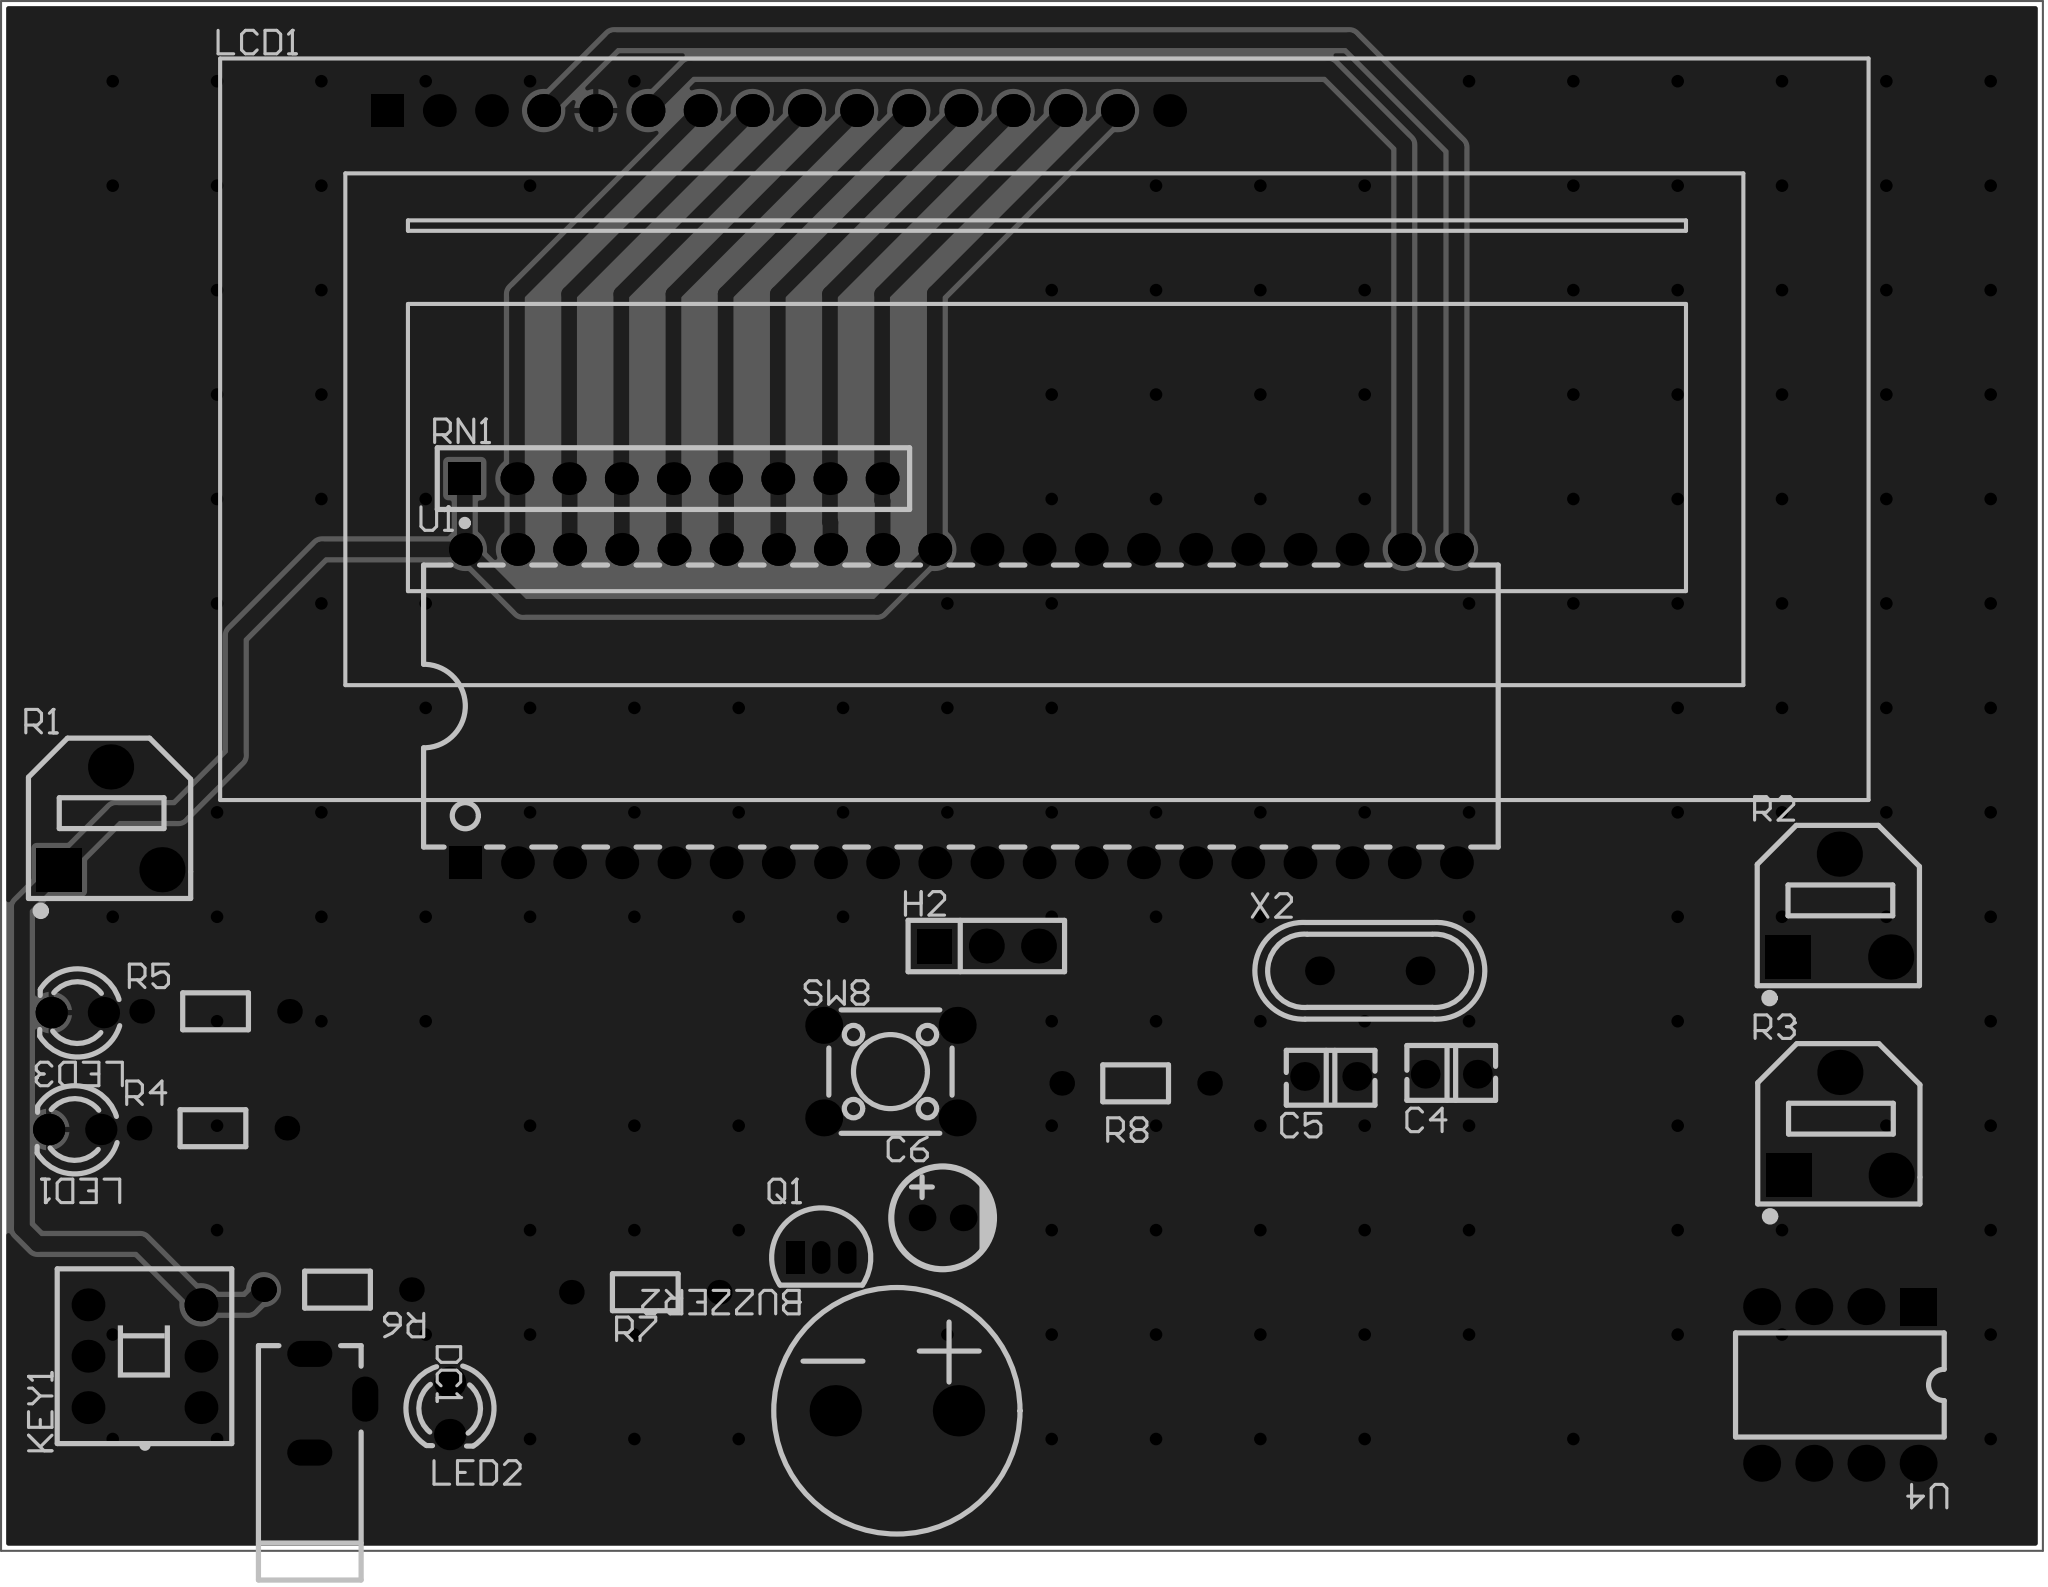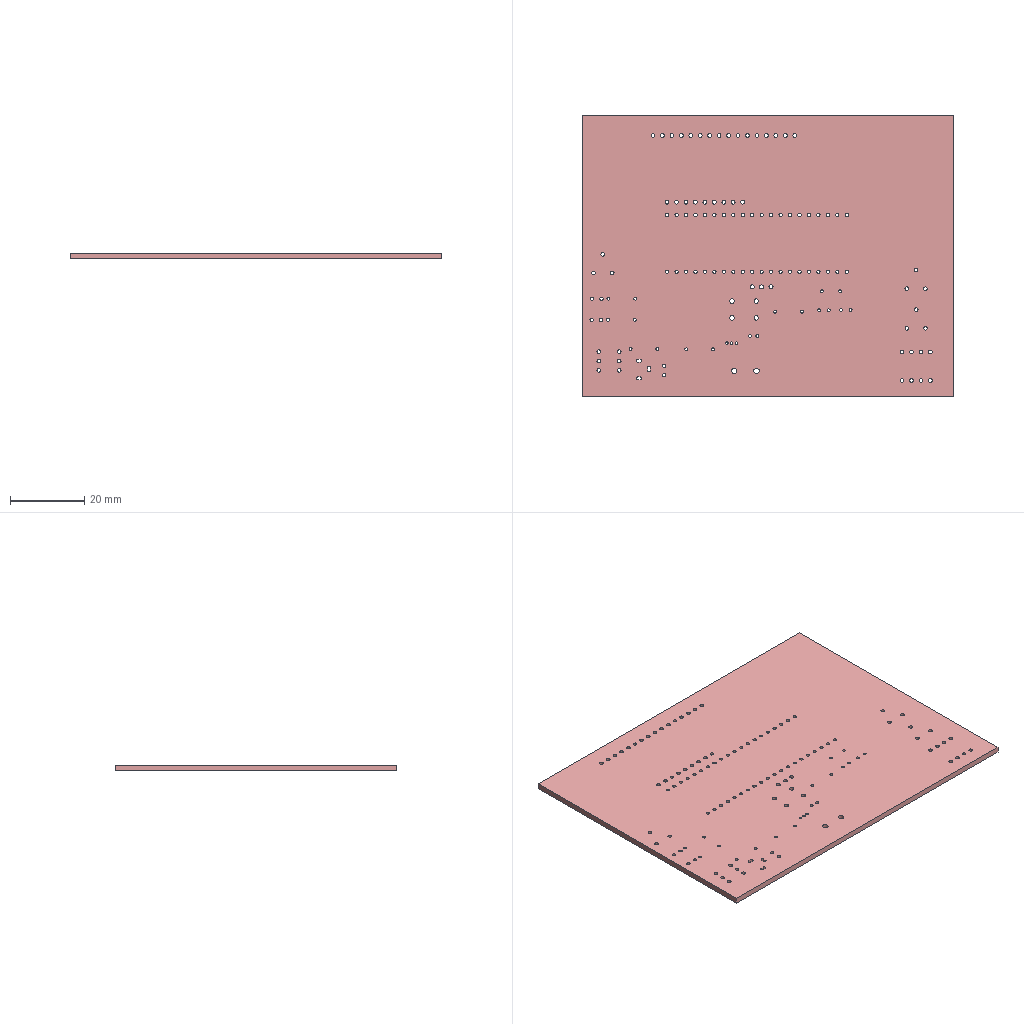Circuit board layout | Altium Designer | box 99.4 x 75.4 x 1.6 mm
Layer stack:
# Altium Designer layer stack of  (unit mm; dielectric type: 0 none, 1 core, 2 prepreg, 3 surface material)
index,name,kind,layer,copper_thickness_mm,dielectric_type,dielectric_thickness_mm,dielectric_material,dielectric_constant
0,Top Paste Mask Layer,other,,,,,,
1,Top Silkscreen Layer,other,,,,,,
2,Top Solder Mask Layer,dielectric,,,3,0.01,,3.3
3,Top Layer,copper,Top Layer,0.035,,,,
4,Dielectric1,dielectric,,,3,1.51,FR4,4.5
5,Bottom Layer,copper,Bottom Layer,0.035,,,,
6,Bottom Solder Mask Layer,dielectric,,,3,0.01,,3.3
7,Bottom Silkscreen Layer,other,,,,,,
8,Bottom Paste Mask Layer,other,,,,,,
# drill layer pairs: low layer,high layer
drill_pair,Top Layer,Bottom Layer
Part placement:
Designator,Comment,Layer,Footprint,Center-X(mm),Center-Y(mm),Rotation
BUZZER2,buzzer,TopLayer,BUZ-TH_BD12.0-P6.00-D0.9-RD,137.346,90.057,0
C4,30pF,TopLayer,CAP-TH_L3.8-W2.5-P2.54-D0.50,164.338,106.426,180
C5,30pF,TopLayer,CAP-TH_L3.8-W2.5-P2.54-D0.50,158.466,106.317,0
C6,10uF,TopLayer,CAP-TH_BD5.0-P2.00-D0.8-FD-10UF50VC110GL,139.573,99.441,0
H2,,TopLayer,HDR-TH_3P-P2.54-V-M,141.702,112.661,0
KEY1,无自锁开关 8.5×8.5 无声,TopLayer,SW-TH_6P-L8.5-W8.5-P2.54,100.711,92.71,90
LCD1,LCD1602,TopLayer,LCD1602,131.576,153.295,0
LED2,,TopLayer,LED_TH-3mm,115.57,90.17,270
R7,1kΩ,TopLayer,Res_1/8W,125.095,95.822,180
R8,10kΩ,TopLayer,Res_1/8W,148.971,105.982,180
R6,1kΩ,TopLayer,Res_1/8W,110.109,95.949,180
SW8,,TopLayer,SW-TH_4P-L6.0-W6.0-P4.50-LS6.5,137.033,106.553,0
U1,STC89C52RC-40I-PDIP40,TopLayer,DIP-40_L52.0-W13.7-P2.54-LS15.2-BL,140.462,124.333,0
X2,11.059MHz,TopLayer,OSC-TH_L11.1-W4.7-P4.88,160.371,111.456,0
DC1,DC-002,TopLayer,DC-IN-TH_DC-3510,110.109,90.424,270
LED1,,TopLayer,LED_TH-3mm,97.314,103.737,180
LED3,,TopLayer,LED_TH-3mm,97.441,109.422,180
Q1,,TopLayer,S8050_TO_92,133.661,97.513,0
R1,10kΩ,TopLayer,RES-ADJ-SMD_RM065-V1,99.06,118.872,0
R2,10kΩ,TopLayer,RES-ADJ-SMD_RM065-V1,183.235,114.629,0
R3,10kΩ,TopLayer,RES-ADJ-SMD_RM065-V1,183.261,104.013,0
R4,220Ω,TopLayer,Res_1/8W,104.045,103.8,0
R5,220Ω,TopLayer,Res_1/8W,104.172,109.485,0
RN1,-,TopLayer,RES-ARRAY-TH_9P-P2.54-D1.0,126.466,135.395,0
U4,XPT2046,TopLayer,DIP-8_L9.7-W6.4-P2.54-LS7.6-BL,183.261,91.313,180
Pad and via stacks:
# Altium Designer via and pad stacks of  (unit mm). Each distinct definition once, with the count of objects using it.
# via: kind,start_layer,end_layer,hole_mm,diameter_mm,mode(0 simple;1 top-mid-bottom;2 full stack),diameter_per_layer,count,example_net
# pad: kind,layer,hole_mm,hole_type(0 round;1 square;2 slot),plating,top_size,top_shape(1 round;2 rect;3 octagon;9 rounded rect),mid_size,bottom_size,mode,footprint,size_per_layer,count,example
pad,Multi-Layer,1.5,0,plated,2.5x2.5,1,2.5x2.5,2.5x2.5,0,BUZ-TH_BD12.0-P6.00-D0.9-RD,,2,BUZZER2.1
pad,Multi-Layer,0.8,0,plated,1.4x1.4,1,1.4x1.4,1.4x1.4,0,CAP-TH_L3.8-W2.5-P2.54-D0.50,,4,C4.1
pad,Multi-Layer,0.8,0,plated,1.3x1.3,1,1.3x1.3,1.3x1.3,0,CAP-TH_BD5.0-P2.00-D0.8-FD-10UF50VC110GL,,2,C6.2
pad,Multi-Layer,1.1,0,plated,1.7x1.7,2,1.7x1.7,1.7x1.7,0,HDR-TH_3P-P2.54-V-M,,1,H2.1
pad,Multi-Layer,1.1,0,plated,1.7x1.7,1,1.7x1.7,1.7x1.7,0,HDR-TH_3P-P2.54-V-M,,2,H2.2
pad,Multi-Layer,1,0,plated,1.6x1.6,1,1.6x1.6,1.6x1.6,0,SW-TH_6P-L8.5-W8.5-P2.54,,6,KEY1.4
pad,Multi-Layer,1,0,plated,1.6x1.6,1,1.6x1.6,1.6x1.6,0,LCD1602,,15,LCD1.16
pad,Multi-Layer,1,0,plated,1.6x1.6,2,1.6x1.6,1.6x1.6,0,LCD1602,,1,LCD1.1
pad,Multi-Layer,0.9144,0,plated,1.524x1.524,1,1.524x1.524,1.524x1.524,0,LED_TH-3mm,,6,LED2.1
pad,Multi-Layer,0.8001,0,plated,1.199x1.199,1,1.199x1.199,1.199x1.199,0,Res_1/8W,,10,R7.1
pad,Multi-Layer,1.2,0,plated,1.8x1.8,1,1.8x1.8,1.8x1.8,0,SW-TH_4P-L6.0-W6.0-P4.50-LS6.5,,4,SW8.1
pad,Multi-Layer,0.889,0,plated,1.6x1.6,1,1.6x1.6,1.6x1.6,0,DIP-40_L52.0-W13.7-P2.54-LS15.2-BL,,39,U1.31
pad,Multi-Layer,0.889,0,plated,1.6x1.6,2,1.6x1.6,1.6x1.6,0,DIP-40_L52.0-W13.7-P2.54-LS15.2-BL,,1,U1.1
pad,Multi-Layer,0.7,0,plated,1.4x1.4,1,1.4x1.4,1.4x1.4,0,OSC-TH_L11.1-W4.7-P4.88,,2,X2.1
pad,Multi-Layer,0.8,2,plated,2.2x1.27,1,2.2x1.27,2.2x1.27,0,DC-IN-TH_DC-3510,,3,DC1.3
pad,Multi-Layer,0.701,0,plated,0.8992x1.6,2,0.8992x1.6,0.8992x1.6,0,S8050_TO_92,,1,Q1.1
pad,Multi-Layer,0.701,0,plated,0.8992x1.6,1,0.8992x1.6,0.8992x1.6,0,S8050_TO_92,,2,Q1.2
pad,Multi-Layer,1,0,plated,2.2x2.1,2,2.2x2.1,2.2x2.1,0,RES-ADJ-SMD_RM065-V1,,3,R1.1
pad,Multi-Layer,1,0,plated,2.2x2.2,1,2.2x2.2,2.2x2.2,0,RES-ADJ-SMD_RM065-V1,,6,R1.3
pad,Multi-Layer,1,0,plated,1.6x1.6,2,1.6x1.6,1.6x1.6,0,RES-ARRAY-TH_9P-P2.54-D1.0,,1,RN1.1
pad,Multi-Layer,1,0,plated,1.6x1.6,1,1.6x1.6,1.6x1.6,0,RES-ARRAY-TH_9P-P2.54-D1.0,,8,RN1.2
pad,Multi-Layer,1,0,plated,1.8x1.8,2,1.8x1.8,1.8x1.8,0,DIP-8_L9.7-W6.4-P2.54-LS7.6-BL,,1,U4.1
pad,Multi-Layer,1,0,plated,1.8x1.8,1,1.8x1.8,1.8x1.8,0,DIP-8_L9.7-W6.4-P2.54-LS7.6-BL,,7,U4.2
via,Top Layer,Bottom Layer,0.3048,0.61,0,,170,GND
Copper pours:
name,layer,net,type(0 solid;1 hatched;2 none)
Bottom Layer-GND,Bottom Layer,GND,0
Top Layer-GND,Top Layer,GND,0
Design rules, without the lines most boards share:
# Altium Designer design rules of  (exported by Altium Designer, unit mm)
# columns: name | kind | enabled | priority | scope1 | scope2 | descriptor | typed fields (field=value)
creepage | 65 | enabled | 1 | All | All | Creepage Distance Constraint =(0mil) (All),(All) |
copperRegion | 20 | enabled | 1 | (InNet('GND')) | All | Polygon Connect Rule(Relief Connect )(Conductor Width=10mil) (Relief Angle=90 Angle) (Entries=4) (Air Gap Width=10mil) ((InNet('GND'))),(All) | connect_style(0=relief,1=direct,2=none)=0 relief_conductor_width=0.254 relief_entries=4